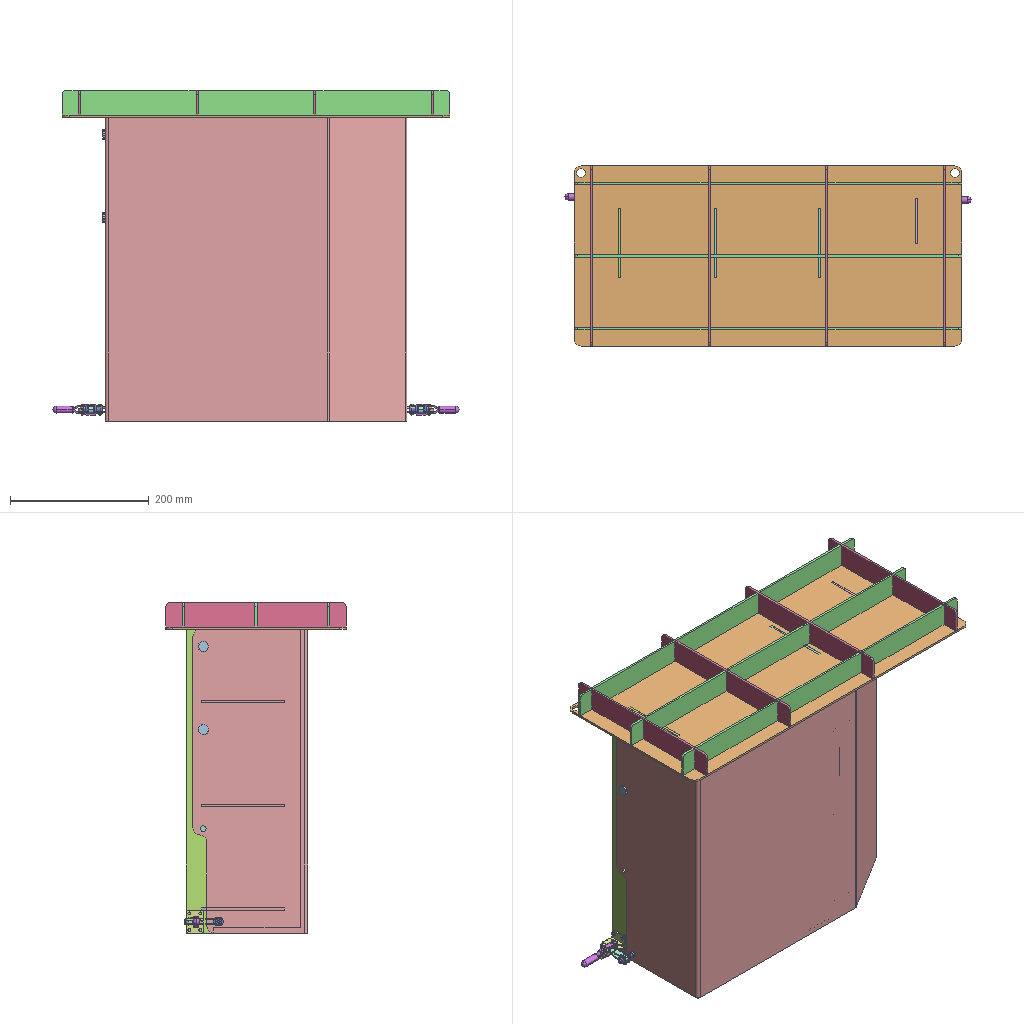Assembly | SolidWorks | 11 different items | 21 placed | box 587 x 260 x 477 mm
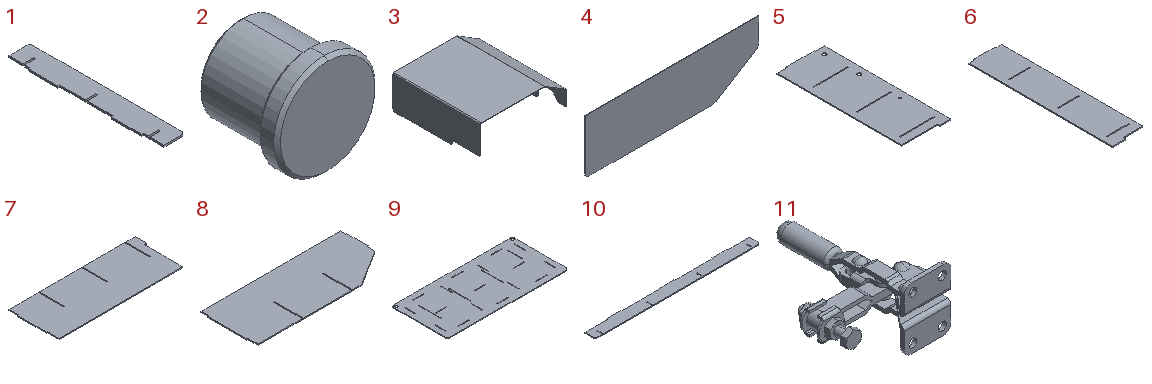Parts list (item | quantity | size | volume | features):
1 | x4 | 38 x 260 x 3.2 mm | 29505 mm3 | features FlatPattern 1, SMBaseFlange 1, SheetMetal 1
2 | x2 | 15 x 13 x 15 mm | 1741 mm3 | features Chamfer 1, Revolution 1
3 | x1 | 436 x 439 x 176 mm | 705533 mm3 | features ICE 2, Fillet 1, FlatPattern 1, SMBaseFlange 1, SheetMetal 1
4 | x1 | 431.35 x 2.3 x 134 mm | 124034 mm3 | features Chamfer 2, FlatPattern 1, SMBaseFlange 1, SheetMetal 1
5 | x1 | 165 x 442 x 3.2 mm | 224791 mm3 | features FlatPattern 1, SMBaseFlange 1, SheetMetal 1
6 | x1 | 100 x 442 x 3.2 mm | 137506 mm3 | features FlatPattern 1, SMBaseFlange 1, SheetMetal 1
7 | x2 | 442 x 173.7 x 3.2 mm | 238742 mm3 | features FlatPattern 1, SMBaseFlange 1, SheetMetal 1
8 | x3 | 431 x 173.7 x 3.2 mm | 224566 mm3 | features FlatPattern 1, SMBaseFlange 1, SheetMetal 1
9 | x1 | 560 x 260 x 3.2 mm | 452354 mm3 | features FlatPattern 1, SMBaseFlange 1, SheetMetal 1
10 | x3 | 560 x 38 x 3.2 mm | 63405 mm3 | features FlatPattern 1, SMBaseFlange 1, SheetMetal 1
11 | x2 | 56.45 x 77.62 x 33.3 mm | 10418 mm3 | features BaseBody 5
Mates (type | each side: item.copy, entity, surface, feature):
DistanceDim | 4.1 face plane Base-Flange1 | 3.1 face plane Base-Flange1
Coincident | 3.1 face plane Base-Flange1 | 4.1 face plane Base-Flange1 | 2 times
InPlace | 3.1 face plane Base-Flange1 | 5.1 plane
InPlace | 3.1 face plane Base-Flange1 | 6.1 plane
InPlace | 7.1 plane | assembly plane
InPlace | 3.1 face plane Base-Flange1 | 9.1 plane
InPlace | 8.1 plane | assembly plane
InPlace | 10.1 plane | assembly plane
InPlace | 1.1 plane | assembly plane
Concentric | 3.1 face cylinder Cut-Extrude1 | 2.1 face cylinder Revolve1
Coincident | 3.1 face plane Base-Flange1 | 2.1 face plane Revolve1
Concentric | 3.1 face cylinder Cut-Extrude1 | 2.2 face cylinder Revolve1
Coincident | 3.1 face plane Base-Flange1 | 2.2 face plane Revolve1
Coincident | 5.1 face plane Base-Flange1 | 11.1 face plane TC1-1 Vertical Flange-Mount Quick Clamp[TCS1-1].step-1/_TCS1-1(seat).step-1-solid1 | 3 times
Coincident | 6.1 face plane Base-Flange1 | 11.2 face plane TC1-1 Vertical Flange-Mount Quick Clamp[TCS1-1].step-1/_TCS1-1(seat).step-1-solid1 | 2 times
Coincident | 3.1 face plane Cut-Extrude2 | 11.2 face plane TC1-1 Vertical Flange-Mount Quick Clamp[TCS1-1].step-1/_TCS1-1(seat).step-1-solid1